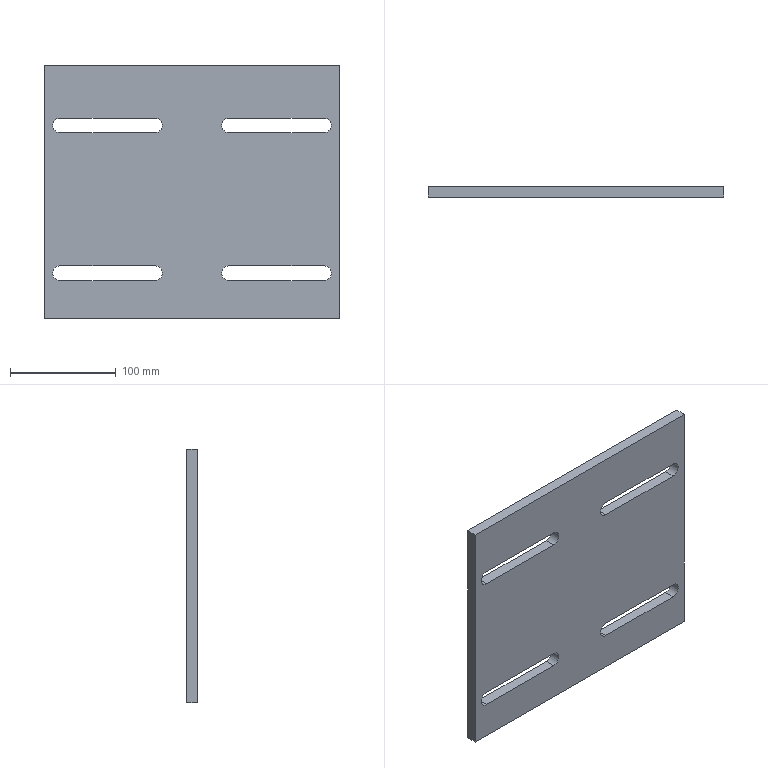Part | STEP file | Produce dryer line heating fan-motor base | 1 solid | 22 faces | box 280 x 10 x 240 mm | volume 615442 mm3 | plane 14 | cylinder 8 | commonest cylinder face diameters 14 x8
STEP:
#1=CARTESIAN_POINT('',(-125.,10.,70.));
#2=VERTEX_POINT('',#1);
#3=CARTESIAN_POINT('',(-35.,10.,70.));
#4=VERTEX_POINT('',#3);
#5=CARTESIAN_POINT('',(-125.,10.,70.));
#6=DIRECTION('',(1.,0.,0.));
#7=VECTOR('',#6,1000.);
#8=LINE('',#5,#7);
#9=EDGE_CURVE('',#2,#4,#8,.T.);
#10=ORIENTED_EDGE('',*,*,#9,.F.);
#11=CARTESIAN_POINT('',(-125.,10.,56.));
#12=VERTEX_POINT('',#11);
#13=CARTESIAN_POINT('',(-125.,10.,63.));
#14=DIRECTION('',(0.,1.,0.));
#15=DIRECTION('',(0.,0.,1.));
#16=AXIS2_PLACEMENT_3D('',#13,#14,#15);
#17=CIRCLE('',#16,7.);
#18=EDGE_CURVE('',#12,#2,#17,.T.);
#19=ORIENTED_EDGE('',*,*,#18,.F.);
#20=CARTESIAN_POINT('',(-35.,10.,56.));
#21=VERTEX_POINT('',#20);
#22=CARTESIAN_POINT('',(-125.,10.,56.));
#23=DIRECTION('',(-1.,0.,0.));
#24=VECTOR('',#23,1000.);
#25=LINE('',#22,#24);
#26=EDGE_CURVE('',#21,#12,#25,.T.);
#27=ORIENTED_EDGE('',*,*,#26,.F.);
#28=CARTESIAN_POINT('',(-35.,10.,63.));
#29=DIRECTION('',(0.,1.,0.));
#30=DIRECTION('',(0.,0.,1.));
#31=AXIS2_PLACEMENT_3D('',#28,#29,#30);
#32=CIRCLE('',#31,7.);
#33=EDGE_CURVE('',#4,#21,#32,.T.);
#34=ORIENTED_EDGE('',*,*,#33,.F.);
#35=EDGE_LOOP('',(#10,#19,#27,#34));
#36=FACE_BOUND('',#35,.T.);
#37=CARTESIAN_POINT('',(-125.,10.,-70.));
#38=VERTEX_POINT('',#37);
#39=CARTESIAN_POINT('',(-35.,10.,-70.));
#40=VERTEX_POINT('',#39);
#41=CARTESIAN_POINT('',(-125.,10.,-70.));
#42=DIRECTION('',(1.,0.,0.));
#43=VECTOR('',#42,1000.);
#44=LINE('',#41,#43);
#45=EDGE_CURVE('',#38,#40,#44,.T.);
#46=ORIENTED_EDGE('',*,*,#45,.F.);
#47=CARTESIAN_POINT('',(-125.,10.,-84.));
#48=VERTEX_POINT('',#47);
#49=CARTESIAN_POINT('',(-125.,10.,-77.));
#50=DIRECTION('',(0.,1.,0.));
#51=DIRECTION('',(0.,0.,1.));
#52=AXIS2_PLACEMENT_3D('',#49,#50,#51);
#53=CIRCLE('',#52,7.);
#54=EDGE_CURVE('',#48,#38,#53,.T.);
#55=ORIENTED_EDGE('',*,*,#54,.F.);
#56=CARTESIAN_POINT('',(-35.,10.,-84.));
#57=VERTEX_POINT('',#56);
#58=CARTESIAN_POINT('',(-125.,10.,-84.));
#59=DIRECTION('',(-1.,0.,0.));
#60=VECTOR('',#59,1000.);
#61=LINE('',#58,#60);
#62=EDGE_CURVE('',#57,#48,#61,.T.);
#63=ORIENTED_EDGE('',*,*,#62,.F.);
#64=CARTESIAN_POINT('',(-35.,10.,-77.));
#65=DIRECTION('',(0.,1.,0.));
#66=DIRECTION('',(0.,0.,1.));
#67=AXIS2_PLACEMENT_3D('',#64,#65,#66);
#68=CIRCLE('',#67,7.);
#69=EDGE_CURVE('',#40,#57,#68,.T.);
#70=ORIENTED_EDGE('',*,*,#69,.F.);
#71=EDGE_LOOP('',(#46,#55,#63,#70));
#72=FACE_BOUND('',#71,.T.);
#73=CARTESIAN_POINT('',(-140.,10.,-120.));
#74=VERTEX_POINT('',#73);
#75=CARTESIAN_POINT('',(-140.,10.,120.));
#76=VERTEX_POINT('',#75);
#77=CARTESIAN_POINT('',(-140.,10.,-120.));
#78=DIRECTION('',(0.,0.,1.));
#79=VECTOR('',#78,1000.);
#80=LINE('',#77,#79);
#81=EDGE_CURVE('',#74,#76,#80,.T.);
#82=ORIENTED_EDGE('',*,*,#81,.T.);
#83=CARTESIAN_POINT('',(140.,10.,120.));
#84=VERTEX_POINT('',#83);
#85=CARTESIAN_POINT('',(-140.,10.,120.));
#86=DIRECTION('',(1.,0.,0.));
#87=VECTOR('',#86,1000.);
#88=LINE('',#85,#87);
#89=EDGE_CURVE('',#76,#84,#88,.T.);
#90=ORIENTED_EDGE('',*,*,#89,.T.);
#91=CARTESIAN_POINT('',(140.,10.,-120.));
#92=VERTEX_POINT('',#91);
#93=CARTESIAN_POINT('',(140.,10.,-120.));
#94=DIRECTION('',(0.,0.,-1.));
#95=VECTOR('',#94,1000.);
#96=LINE('',#93,#95);
#97=EDGE_CURVE('',#84,#92,#96,.T.);
#98=ORIENTED_EDGE('',*,*,#97,.T.);
#99=CARTESIAN_POINT('',(-140.,10.,-120.));
#100=DIRECTION('',(-1.,0.,0.));
#101=VECTOR('',#100,1000.);
#102=LINE('',#99,#101);
#103=EDGE_CURVE('',#92,#74,#102,.T.);
#104=ORIENTED_EDGE('',*,*,#103,.T.);
#105=EDGE_LOOP('',(#82,#90,#98,#104));
#106=FACE_OUTER_BOUND('',#105,.T.);
#107=CARTESIAN_POINT('',(125.,10.,-84.));
#108=VERTEX_POINT('',#107);
#109=CARTESIAN_POINT('',(35.,10.,-84.));
#110=VERTEX_POINT('',#109);
#111=CARTESIAN_POINT('',(125.,10.,-84.));
#112=DIRECTION('',(-1.,0.,0.));
#113=VECTOR('',#112,1000.);
#114=LINE('',#111,#113);
#115=EDGE_CURVE('',#108,#110,#114,.T.);
#116=ORIENTED_EDGE('',*,*,#115,.F.);
#117=CARTESIAN_POINT('',(125.,10.,-70.));
#118=VERTEX_POINT('',#117);
#119=CARTESIAN_POINT('',(125.,10.,-77.));
#120=DIRECTION('',(0.,1.,0.));
#121=DIRECTION('',(0.,0.,1.));
#122=AXIS2_PLACEMENT_3D('',#119,#120,#121);
#123=CIRCLE('',#122,7.);
#124=EDGE_CURVE('',#118,#108,#123,.T.);
#125=ORIENTED_EDGE('',*,*,#124,.F.);
#126=CARTESIAN_POINT('',(35.,10.,-70.));
#127=VERTEX_POINT('',#126);
#128=CARTESIAN_POINT('',(125.,10.,-70.));
#129=DIRECTION('',(1.,0.,0.));
#130=VECTOR('',#129,1000.);
#131=LINE('',#128,#130);
#132=EDGE_CURVE('',#127,#118,#131,.T.);
#133=ORIENTED_EDGE('',*,*,#132,.F.);
#134=CARTESIAN_POINT('',(35.,10.,-77.));
#135=DIRECTION('',(0.,1.,0.));
#136=DIRECTION('',(0.,0.,1.));
#137=AXIS2_PLACEMENT_3D('',#134,#135,#136);
#138=CIRCLE('',#137,7.);
#139=EDGE_CURVE('',#110,#127,#138,.T.);
#140=ORIENTED_EDGE('',*,*,#139,.F.);
#141=EDGE_LOOP('',(#116,#125,#133,#140));
#142=FACE_BOUND('',#141,.T.);
#143=CARTESIAN_POINT('',(35.,10.,70.));
#144=VERTEX_POINT('',#143);
#145=CARTESIAN_POINT('',(125.,10.,70.));
#146=VERTEX_POINT('',#145);
#147=CARTESIAN_POINT('',(35.,10.,70.));
#148=DIRECTION('',(1.,0.,0.));
#149=VECTOR('',#148,1000.);
#150=LINE('',#147,#149);
#151=EDGE_CURVE('',#144,#146,#150,.T.);
#152=ORIENTED_EDGE('',*,*,#151,.F.);
#153=CARTESIAN_POINT('',(35.,10.,56.));
#154=VERTEX_POINT('',#153);
#155=CARTESIAN_POINT('',(35.,10.,63.));
#156=DIRECTION('',(0.,1.,0.));
#157=DIRECTION('',(0.,0.,1.));
#158=AXIS2_PLACEMENT_3D('',#155,#156,#157);
#159=CIRCLE('',#158,7.);
#160=EDGE_CURVE('',#154,#144,#159,.T.);
#161=ORIENTED_EDGE('',*,*,#160,.F.);
#162=CARTESIAN_POINT('',(125.,10.,56.));
#163=VERTEX_POINT('',#162);
#164=CARTESIAN_POINT('',(35.,10.,56.));
#165=DIRECTION('',(-1.,0.,0.));
#166=VECTOR('',#165,1000.);
#167=LINE('',#164,#166);
#168=EDGE_CURVE('',#163,#154,#167,.T.);
#169=ORIENTED_EDGE('',*,*,#168,.F.);
#170=CARTESIAN_POINT('',(125.,10.,63.));
#171=DIRECTION('',(0.,1.,0.));
#172=DIRECTION('',(0.,0.,1.));
#173=AXIS2_PLACEMENT_3D('',#170,#171,#172);
#174=CIRCLE('',#173,7.);
#175=EDGE_CURVE('',#146,#163,#174,.T.);
#176=ORIENTED_EDGE('',*,*,#175,.F.);
#177=EDGE_LOOP('',(#152,#161,#169,#176));
#178=FACE_BOUND('',#177,.T.);
#179=CARTESIAN_POINT('',(-140.,10.,120.));
#180=DIRECTION('',(0.,1.,0.));
#181=DIRECTION('',(0.,0.,1.));
#182=AXIS2_PLACEMENT_3D('',#179,#180,#181);
#183=PLANE('',#182);
#184=ADVANCED_FACE('',(#36,#72,#106,#142,#178),#183,.T.);
#185=CARTESIAN_POINT('',(-125.,0.,56.));
#186=VERTEX_POINT('',#185);
#187=CARTESIAN_POINT('',(-125.,0.,70.));
#188=VERTEX_POINT('',#187);
#189=CARTESIAN_POINT('',(-125.,0.,63.));
#190=DIRECTION('',(0.,1.,0.));
#191=DIRECTION('',(0.,0.,1.));
#192=AXIS2_PLACEMENT_3D('',#189,#190,#191);
#193=CIRCLE('',#192,7.);
#194=EDGE_CURVE('',#186,#188,#193,.T.);
#195=ORIENTED_EDGE('',*,*,#194,.T.);
#196=CARTESIAN_POINT('',(-35.,0.,70.));
#197=VERTEX_POINT('',#196);
#198=CARTESIAN_POINT('',(-125.,0.,70.));
#199=DIRECTION('',(1.,0.,0.));
#200=VECTOR('',#199,1000.);
#201=LINE('',#198,#200);
#202=EDGE_CURVE('',#188,#197,#201,.T.);
#203=ORIENTED_EDGE('',*,*,#202,.T.);
#204=CARTESIAN_POINT('',(-35.,0.,56.));
#205=VERTEX_POINT('',#204);
#206=CARTESIAN_POINT('',(-35.,0.,63.));
#207=DIRECTION('',(0.,1.,0.));
#208=DIRECTION('',(0.,0.,1.));
#209=AXIS2_PLACEMENT_3D('',#206,#207,#208);
#210=CIRCLE('',#209,7.);
#211=EDGE_CURVE('',#197,#205,#210,.T.);
#212=ORIENTED_EDGE('',*,*,#211,.T.);
#213=CARTESIAN_POINT('',(-125.,0.,56.));
#214=DIRECTION('',(-1.,0.,0.));
#215=VECTOR('',#214,1000.);
#216=LINE('',#213,#215);
#217=EDGE_CURVE('',#205,#186,#216,.T.);
#218=ORIENTED_EDGE('',*,*,#217,.T.);
#219=EDGE_LOOP('',(#195,#203,#212,#218));
#220=FACE_BOUND('',#219,.T.);
#221=CARTESIAN_POINT('',(-125.,0.,-84.));
#222=VERTEX_POINT('',#221);
#223=CARTESIAN_POINT('',(-125.,0.,-70.));
#224=VERTEX_POINT('',#223);
#225=CARTESIAN_POINT('',(-125.,0.,-77.));
#226=DIRECTION('',(0.,1.,0.));
#227=DIRECTION('',(0.,0.,1.));
#228=AXIS2_PLACEMENT_3D('',#225,#226,#227);
#229=CIRCLE('',#228,7.);
#230=EDGE_CURVE('',#222,#224,#229,.T.);
#231=ORIENTED_EDGE('',*,*,#230,.T.);
#232=CARTESIAN_POINT('',(-35.,0.,-70.));
#233=VERTEX_POINT('',#232);
#234=CARTESIAN_POINT('',(-125.,0.,-70.));
#235=DIRECTION('',(1.,0.,0.));
#236=VECTOR('',#235,1000.);
#237=LINE('',#234,#236);
#238=EDGE_CURVE('',#224,#233,#237,.T.);
#239=ORIENTED_EDGE('',*,*,#238,.T.);
#240=CARTESIAN_POINT('',(-35.,0.,-84.));
#241=VERTEX_POINT('',#240);
#242=CARTESIAN_POINT('',(-35.,0.,-77.));
#243=DIRECTION('',(0.,1.,0.));
#244=DIRECTION('',(0.,0.,1.));
#245=AXIS2_PLACEMENT_3D('',#242,#243,#244);
#246=CIRCLE('',#245,7.);
#247=EDGE_CURVE('',#233,#241,#246,.T.);
#248=ORIENTED_EDGE('',*,*,#247,.T.);
#249=CARTESIAN_POINT('',(-125.,0.,-84.));
#250=DIRECTION('',(-1.,0.,0.));
#251=VECTOR('',#250,1000.);
#252=LINE('',#249,#251);
#253=EDGE_CURVE('',#241,#222,#252,.T.);
#254=ORIENTED_EDGE('',*,*,#253,.T.);
#255=EDGE_LOOP('',(#231,#239,#248,#254));
#256=FACE_BOUND('',#255,.T.);
#257=CARTESIAN_POINT('',(-140.,0.,-120.));
#258=VERTEX_POINT('',#257);
#259=CARTESIAN_POINT('',(-140.,0.,120.));
#260=VERTEX_POINT('',#259);
#261=CARTESIAN_POINT('',(-140.,0.,-120.));
#262=DIRECTION('',(0.,0.,1.));
#263=VECTOR('',#262,1000.);
#264=LINE('',#261,#263);
#265=EDGE_CURVE('',#258,#260,#264,.T.);
#266=ORIENTED_EDGE('',*,*,#265,.F.);
#267=CARTESIAN_POINT('',(140.,0.,-120.));
#268=VERTEX_POINT('',#267);
#269=CARTESIAN_POINT('',(-140.,0.,-120.));
#270=DIRECTION('',(-1.,0.,0.));
#271=VECTOR('',#270,1000.);
#272=LINE('',#269,#271);
#273=EDGE_CURVE('',#268,#258,#272,.T.);
#274=ORIENTED_EDGE('',*,*,#273,.F.);
#275=CARTESIAN_POINT('',(140.,0.,120.));
#276=VERTEX_POINT('',#275);
#277=CARTESIAN_POINT('',(140.,0.,-120.));
#278=DIRECTION('',(0.,0.,-1.));
#279=VECTOR('',#278,1000.);
#280=LINE('',#277,#279);
#281=EDGE_CURVE('',#276,#268,#280,.T.);
#282=ORIENTED_EDGE('',*,*,#281,.F.);
#283=CARTESIAN_POINT('',(-140.,0.,120.));
#284=DIRECTION('',(1.,0.,0.));
#285=VECTOR('',#284,1000.);
#286=LINE('',#283,#285);
#287=EDGE_CURVE('',#260,#276,#286,.T.);
#288=ORIENTED_EDGE('',*,*,#287,.F.);
#289=EDGE_LOOP('',(#266,#274,#282,#288));
#290=FACE_OUTER_BOUND('',#289,.T.);
#291=CARTESIAN_POINT('',(125.,0.,-70.));
#292=VERTEX_POINT('',#291);
#293=CARTESIAN_POINT('',(125.,0.,-84.));
#294=VERTEX_POINT('',#293);
#295=CARTESIAN_POINT('',(125.,0.,-77.));
#296=DIRECTION('',(0.,1.,0.));
#297=DIRECTION('',(0.,0.,1.));
#298=AXIS2_PLACEMENT_3D('',#295,#296,#297);
#299=CIRCLE('',#298,7.);
#300=EDGE_CURVE('',#292,#294,#299,.T.);
#301=ORIENTED_EDGE('',*,*,#300,.T.);
#302=CARTESIAN_POINT('',(35.,0.,-84.));
#303=VERTEX_POINT('',#302);
#304=CARTESIAN_POINT('',(125.,0.,-84.));
#305=DIRECTION('',(-1.,0.,0.));
#306=VECTOR('',#305,1000.);
#307=LINE('',#304,#306);
#308=EDGE_CURVE('',#294,#303,#307,.T.);
#309=ORIENTED_EDGE('',*,*,#308,.T.);
#310=CARTESIAN_POINT('',(35.,0.,-70.));
#311=VERTEX_POINT('',#310);
#312=CARTESIAN_POINT('',(35.,0.,-77.));
#313=DIRECTION('',(0.,1.,0.));
#314=DIRECTION('',(0.,0.,1.));
#315=AXIS2_PLACEMENT_3D('',#312,#313,#314);
#316=CIRCLE('',#315,7.);
#317=EDGE_CURVE('',#303,#311,#316,.T.);
#318=ORIENTED_EDGE('',*,*,#317,.T.);
#319=CARTESIAN_POINT('',(125.,0.,-70.));
#320=DIRECTION('',(1.,0.,0.));
#321=VECTOR('',#320,1000.);
#322=LINE('',#319,#321);
#323=EDGE_CURVE('',#311,#292,#322,.T.);
#324=ORIENTED_EDGE('',*,*,#323,.T.);
#325=EDGE_LOOP('',(#301,#309,#318,#324));
#326=FACE_BOUND('',#325,.T.);
#327=CARTESIAN_POINT('',(35.,0.,56.));
#328=VERTEX_POINT('',#327);
#329=CARTESIAN_POINT('',(35.,0.,70.));
#330=VERTEX_POINT('',#329);
#331=CARTESIAN_POINT('',(35.,0.,63.));
#332=DIRECTION('',(0.,1.,0.));
#333=DIRECTION('',(0.,0.,1.));
#334=AXIS2_PLACEMENT_3D('',#331,#332,#333);
#335=CIRCLE('',#334,7.);
#336=EDGE_CURVE('',#328,#330,#335,.T.);
#337=ORIENTED_EDGE('',*,*,#336,.T.);
#338=CARTESIAN_POINT('',(125.,0.,70.));
#339=VERTEX_POINT('',#338);
#340=CARTESIAN_POINT('',(35.,0.,70.));
#341=DIRECTION('',(1.,0.,0.));
#342=VECTOR('',#341,1000.);
#343=LINE('',#340,#342);
#344=EDGE_CURVE('',#330,#339,#343,.T.);
#345=ORIENTED_EDGE('',*,*,#344,.T.);
#346=CARTESIAN_POINT('',(125.,0.,56.));
#347=VERTEX_POINT('',#346);
#348=CARTESIAN_POINT('',(125.,0.,63.));
#349=DIRECTION('',(0.,1.,0.));
#350=DIRECTION('',(0.,0.,1.));
#351=AXIS2_PLACEMENT_3D('',#348,#349,#350);
#352=CIRCLE('',#351,7.);
#353=EDGE_CURVE('',#339,#347,#352,.T.);
#354=ORIENTED_EDGE('',*,*,#353,.T.);
#355=CARTESIAN_POINT('',(35.,0.,56.));
#356=DIRECTION('',(-1.,0.,0.));
#357=VECTOR('',#356,1000.);
#358=LINE('',#355,#357);
#359=EDGE_CURVE('',#347,#328,#358,.T.);
#360=ORIENTED_EDGE('',*,*,#359,.T.);
#361=EDGE_LOOP('',(#337,#345,#354,#360));
#362=FACE_BOUND('',#361,.T.);
#363=CARTESIAN_POINT('',(-140.,0.,120.));
#364=DIRECTION('',(0.,1.,0.));
#365=DIRECTION('',(0.,0.,1.));
#366=AXIS2_PLACEMENT_3D('',#363,#364,#365);
#367=PLANE('',#366);
#368=ADVANCED_FACE('',(#220,#256,#290,#326,#362),#367,.F.);
#369=ORIENTED_EDGE('',*,*,#265,.T.);
#370=CARTESIAN_POINT('',(-140.,10.,120.));
#371=DIRECTION('',(0.,-1.,0.));
#372=VECTOR('',#371,1000.);
#373=LINE('',#370,#372);
#374=EDGE_CURVE('',#76,#260,#373,.T.);
#375=ORIENTED_EDGE('',*,*,#374,.F.);
#376=ORIENTED_EDGE('',*,*,#81,.F.);
#377=CARTESIAN_POINT('',(-140.,10.,-120.));
#378=DIRECTION('',(0.,-1.,0.));
#379=VECTOR('',#378,1000.);
#380=LINE('',#377,#379);
#381=EDGE_CURVE('',#74,#258,#380,.T.);
#382=ORIENTED_EDGE('',*,*,#381,.T.);
#383=EDGE_LOOP('',(#369,#375,#376,#382));
#384=FACE_OUTER_BOUND('',#383,.T.);
#385=CARTESIAN_POINT('',(-140.,10.,-120.));
#386=DIRECTION('',(1.,0.,0.));
#387=DIRECTION('',(0.,0.,-1.));
#388=AXIS2_PLACEMENT_3D('',#385,#386,#387);
#389=PLANE('',#388);
#390=ADVANCED_FACE('',(#384),#389,.F.);
#391=ORIENTED_EDGE('',*,*,#287,.T.);
#392=CARTESIAN_POINT('',(140.,10.,120.));
#393=DIRECTION('',(0.,-1.,0.));
#394=VECTOR('',#393,1000.);
#395=LINE('',#392,#394);
#396=EDGE_CURVE('',#84,#276,#395,.T.);
#397=ORIENTED_EDGE('',*,*,#396,.F.);
#398=ORIENTED_EDGE('',*,*,#89,.F.);
#399=ORIENTED_EDGE('',*,*,#374,.T.);
#400=EDGE_LOOP('',(#391,#397,#398,#399));
#401=FACE_OUTER_BOUND('',#400,.T.);
#402=CARTESIAN_POINT('',(-140.,10.,120.));
#403=DIRECTION('',(0.,0.,-1.));
#404=DIRECTION('',(-1.,0.,0.));
#405=AXIS2_PLACEMENT_3D('',#402,#403,#404);
#406=PLANE('',#405);
#407=ADVANCED_FACE('',(#401),#406,.F.);
#408=ORIENTED_EDGE('',*,*,#281,.T.);
#409=CARTESIAN_POINT('',(140.,10.,-120.));
#410=DIRECTION('',(0.,-1.,0.));
#411=VECTOR('',#410,1000.);
#412=LINE('',#409,#411);
#413=EDGE_CURVE('',#92,#268,#412,.T.);
#414=ORIENTED_EDGE('',*,*,#413,.F.);
#415=ORIENTED_EDGE('',*,*,#97,.F.);
#416=ORIENTED_EDGE('',*,*,#396,.T.);
#417=EDGE_LOOP('',(#408,#414,#415,#416));
#418=FACE_OUTER_BOUND('',#417,.T.);
#419=CARTESIAN_POINT('',(140.,10.,-120.));
#420=DIRECTION('',(-1.,0.,0.));
#421=DIRECTION('',(0.,0.,1.));
#422=AXIS2_PLACEMENT_3D('',#419,#420,#421);
#423=PLANE('',#422);
#424=ADVANCED_FACE('',(#418),#423,.F.);
#425=ORIENTED_EDGE('',*,*,#273,.T.);
#426=ORIENTED_EDGE('',*,*,#381,.F.);
#427=ORIENTED_EDGE('',*,*,#103,.F.);
#428=ORIENTED_EDGE('',*,*,#413,.T.);
#429=EDGE_LOOP('',(#425,#426,#427,#428));
#430=FACE_OUTER_BOUND('',#429,.T.);
#431=CARTESIAN_POINT('',(-140.,10.,-120.));
#432=DIRECTION('',(0.,0.,1.));
#433=DIRECTION('',(1.,0.,0.));
#434=AXIS2_PLACEMENT_3D('',#431,#432,#433);
#435=PLANE('',#434);
#436=ADVANCED_FACE('',(#430),#435,.F.);
#437=ORIENTED_EDGE('',*,*,#230,.F.);
#438=CARTESIAN_POINT('',(-125.,10.,-84.));
#439=DIRECTION('',(0.,-1.,0.));
#440=VECTOR('',#439,1000.);
#441=LINE('',#438,#440);
#442=EDGE_CURVE('',#48,#222,#441,.T.);
#443=ORIENTED_EDGE('',*,*,#442,.F.);
#444=ORIENTED_EDGE('',*,*,#54,.T.);
#445=CARTESIAN_POINT('',(-125.,10.,-70.));
#446=DIRECTION('',(0.,-1.,0.));
#447=VECTOR('',#446,1000.);
#448=LINE('',#445,#447);
#449=EDGE_CURVE('',#38,#224,#448,.T.);
#450=ORIENTED_EDGE('',*,*,#449,.T.);
#451=EDGE_LOOP('',(#437,#443,#444,#450));
#452=FACE_OUTER_BOUND('',#451,.T.);
#453=CARTESIAN_POINT('',(-125.,10.,-77.));
#454=DIRECTION('',(0.,-1.,0.));
#455=DIRECTION('',(0.,0.,-1.));
#456=AXIS2_PLACEMENT_3D('',#453,#454,#455);
#457=CYLINDRICAL_SURFACE('',#456,7.);
#458=ADVANCED_FACE('',(#452),#457,.F.);
#459=ORIENTED_EDGE('',*,*,#238,.F.);
#460=ORIENTED_EDGE('',*,*,#449,.F.);
#461=ORIENTED_EDGE('',*,*,#45,.T.);
#462=CARTESIAN_POINT('',(-35.,10.,-70.));
#463=DIRECTION('',(0.,-1.,0.));
#464=VECTOR('',#463,1000.);
#465=LINE('',#462,#464);
#466=EDGE_CURVE('',#40,#233,#465,.T.);
#467=ORIENTED_EDGE('',*,*,#466,.T.);
#468=EDGE_LOOP('',(#459,#460,#461,#467));
#469=FACE_OUTER_BOUND('',#468,.T.);
#470=CARTESIAN_POINT('',(-125.,10.,-70.));
#471=DIRECTION('',(0.,0.,-1.));
#472=DIRECTION('',(-1.,0.,0.));
#473=AXIS2_PLACEMENT_3D('',#470,#471,#472);
#474=PLANE('',#473);
#475=ADVANCED_FACE('',(#469),#474,.T.);
#476=ORIENTED_EDGE('',*,*,#247,.F.);
#477=ORIENTED_EDGE('',*,*,#466,.F.);
#478=ORIENTED_EDGE('',*,*,#69,.T.);
#479=CARTESIAN_POINT('',(-35.,10.,-84.));
#480=DIRECTION('',(0.,-1.,0.));
#481=VECTOR('',#480,1000.);
#482=LINE('',#479,#481);
#483=EDGE_CURVE('',#57,#241,#482,.T.);
#484=ORIENTED_EDGE('',*,*,#483,.T.);
#485=EDGE_LOOP('',(#476,#477,#478,#484));
#486=FACE_OUTER_BOUND('',#485,.T.);
#487=CARTESIAN_POINT('',(-35.,10.,-77.));
#488=DIRECTION('',(0.,-1.,0.));
#489=DIRECTION('',(0.,0.,-1.));
#490=AXIS2_PLACEMENT_3D('',#487,#488,#489);
#491=CYLINDRICAL_SURFACE('',#490,7.);
#492=ADVANCED_FACE('',(#486),#491,.F.);
#493=ORIENTED_EDGE('',*,*,#253,.F.);
#494=ORIENTED_EDGE('',*,*,#483,.F.);
#495=ORIENTED_EDGE('',*,*,#62,.T.);
#496=ORIENTED_EDGE('',*,*,#442,.T.);
#497=EDGE_LOOP('',(#493,#494,#495,#496));
#498=FACE_OUTER_BOUND('',#497,.T.);
#499=CARTESIAN_POINT('',(-125.,10.,-84.));
#500=DIRECTION('',(0.,0.,1.));
#501=DIRECTION('',(1.,0.,0.));
#502=AXIS2_PLACEMENT_3D('',#499,#500,#501);
#503=PLANE('',#502);
#504=ADVANCED_FACE('',(#498),#503,.T.);
#505=ORIENTED_EDGE('',*,*,#300,.F.);
#506=CARTESIAN_POINT('',(125.,10.,-70.));
#507=DIRECTION('',(0.,-1.,0.));
#508=VECTOR('',#507,1000.);
#509=LINE('',#506,#508);
#510=EDGE_CURVE('',#118,#292,#509,.T.);
#511=ORIENTED_EDGE('',*,*,#510,.F.);
#512=ORIENTED_EDGE('',*,*,#124,.T.);
#513=CARTESIAN_POINT('',(125.,10.,-84.));
#514=DIRECTION('',(0.,-1.,0.));
#515=VECTOR('',#514,1000.);
#516=LINE('',#513,#515);
#517=EDGE_CURVE('',#108,#294,#516,.T.);
#518=ORIENTED_EDGE('',*,*,#517,.T.);
#519=EDGE_LOOP('',(#505,#511,#512,#518));
#520=FACE_OUTER_BOUND('',#519,.T.);
#521=CARTESIAN_POINT('',(125.,10.,-77.));
#522=DIRECTION('',(0.,-1.,0.));
#523=DIRECTION('',(0.,0.,-1.));
#524=AXIS2_PLACEMENT_3D('',#521,#522,#523);
#525=CYLINDRICAL_SURFACE('',#524,7.);
#526=ADVANCED_FACE('',(#520),#525,.F.);
#527=ORIENTED_EDGE('',*,*,#308,.F.);
#528=ORIENTED_EDGE('',*,*,#517,.F.);
#529=ORIENTED_EDGE('',*,*,#115,.T.);
#530=CARTESIAN_POINT('',(35.,10.,-84.));
#531=DIRECTION('',(0.,-1.,0.));
#532=VECTOR('',#531,1000.);
#533=LINE('',#530,#532);
#534=EDGE_CURVE('',#110,#303,#533,.T.);
#535=ORIENTED_EDGE('',*,*,#534,.T.);
#536=EDGE_LOOP('',(#527,#528,#529,#535));
#537=FACE_OUTER_BOUND('',#536,.T.);
#538=CARTESIAN_POINT('',(125.,10.,-84.));
#539=DIRECTION('',(0.,0.,1.));
#540=DIRECTION('',(1.,0.,0.));
#541=AXIS2_PLACEMENT_3D('',#538,#539,#540);
#542=PLANE('',#541);
#543=ADVANCED_FACE('',(#537),#542,.T.);
#544=ORIENTED_EDGE('',*,*,#317,.F.);
#545=ORIENTED_EDGE('',*,*,#534,.F.);
#546=ORIENTED_EDGE('',*,*,#139,.T.);
#547=CARTESIAN_POINT('',(35.,10.,-70.));
#548=DIRECTION('',(0.,-1.,0.));
#549=VECTOR('',#548,1000.);
#550=LINE('',#547,#549);
#551=EDGE_CURVE('',#127,#311,#550,.T.);
#552=ORIENTED_EDGE('',*,*,#551,.T.);
#553=EDGE_LOOP('',(#544,#545,#546,#552));
#554=FACE_OUTER_BOUND('',#553,.T.);
#555=CARTESIAN_POINT('',(35.,10.,-77.));
#556=DIRECTION('',(0.,-1.,0.));
#557=DIRECTION('',(0.,0.,-1.));
#558=AXIS2_PLACEMENT_3D('',#555,#556,#557);
#559=CYLINDRICAL_SURFACE('',#558,7.);
#560=ADVANCED_FACE('',(#554),#559,.F.);
#561=ORIENTED_EDGE('',*,*,#323,.F.);
#562=ORIENTED_EDGE('',*,*,#551,.F.);
#563=ORIENTED_EDGE('',*,*,#132,.T.);
#564=ORIENTED_EDGE('',*,*,#510,.T.);
#565=EDGE_LOOP('',(#561,#562,#563,#564));
#566=FACE_OUTER_BOUND('',#565,.T.);
#567=CARTESIAN_POINT('',(125.,10.,-70.));
#568=DIRECTION('',(0.,0.,-1.));
#569=DIRECTION('',(-1.,0.,0.));
#570=AXIS2_PLACEMENT_3D('',#567,#568,#569);
#571=PLANE('',#570);
#572=ADVANCED_FACE('',(#566),#571,.T.);
#573=ORIENTED_EDGE('',*,*,#194,.F.);
#574=CARTESIAN_POINT('',(-125.,10.,56.));
#575=DIRECTION('',(0.,-1.,0.));
#576=VECTOR('',#575,1000.);
#577=LINE('',#574,#576);
#578=EDGE_CURVE('',#12,#186,#577,.T.);
#579=ORIENTED_EDGE('',*,*,#578,.F.);
#580=ORIENTED_EDGE('',*,*,#18,.T.);
#581=CARTESIAN_POINT('',(-125.,10.,70.));
#582=DIRECTION('',(0.,-1.,0.));
#583=VECTOR('',#582,1000.);
#584=LINE('',#581,#583);
#585=EDGE_CURVE('',#2,#188,#584,.T.);
#586=ORIENTED_EDGE('',*,*,#585,.T.);
#587=EDGE_LOOP('',(#573,#579,#580,#586));
#588=FACE_OUTER_BOUND('',#587,.T.);
#589=CARTESIAN_POINT('',(-125.,10.,63.));
#590=DIRECTION('',(0.,-1.,0.));
#591=DIRECTION('',(0.,0.,-1.));
#592=AXIS2_PLACEMENT_3D('',#589,#590,#591);
#593=CYLINDRICAL_SURFACE('',#592,7.);
#594=ADVANCED_FACE('',(#588),#593,.F.);
#595=ORIENTED_EDGE('',*,*,#202,.F.);
#596=ORIENTED_EDGE('',*,*,#585,.F.);
#597=ORIENTED_EDGE('',*,*,#9,.T.);
#598=CARTESIAN_POINT('',(-35.,10.,70.));
#599=DIRECTION('',(0.,-1.,0.));
#600=VECTOR('',#599,1000.);
#601=LINE('',#598,#600);
#602=EDGE_CURVE('',#4,#197,#601,.T.);
#603=ORIENTED_EDGE('',*,*,#602,.T.);
#604=EDGE_LOOP('',(#595,#596,#597,#603));
#605=FACE_OUTER_BOUND('',#604,.T.);
#606=CARTESIAN_POINT('',(-125.,10.,70.));
#607=DIRECTION('',(0.,0.,-1.));
#608=DIRECTION('',(-1.,0.,0.));
#609=AXIS2_PLACEMENT_3D('',#606,#607,#608);
#610=PLANE('',#609);
#611=ADVANCED_FACE('',(#605),#610,.T.);
#612=ORIENTED_EDGE('',*,*,#211,.F.);
#613=ORIENTED_EDGE('',*,*,#602,.F.);
#614=ORIENTED_EDGE('',*,*,#33,.T.);
#615=CARTESIAN_POINT('',(-35.,10.,56.));
#616=DIRECTION('',(0.,-1.,0.));
#617=VECTOR('',#616,1000.);
#618=LINE('',#615,#617);
#619=EDGE_CURVE('',#21,#205,#618,.T.);
#620=ORIENTED_EDGE('',*,*,#619,.T.);
#621=EDGE_LOOP('',(#612,#613,#614,#620));
#622=FACE_OUTER_BOUND('',#621,.T.);
#623=CARTESIAN_POINT('',(-35.,10.,63.));
#624=DIRECTION('',(0.,-1.,0.));
#625=DIRECTION('',(0.,0.,-1.));
#626=AXIS2_PLACEMENT_3D('',#623,#624,#625);
#627=CYLINDRICAL_SURFACE('',#626,7.);
#628=ADVANCED_FACE('',(#622),#627,.F.);
#629=ORIENTED_EDGE('',*,*,#217,.F.);
#630=ORIENTED_EDGE('',*,*,#619,.F.);
#631=ORIENTED_EDGE('',*,*,#26,.T.);
#632=ORIENTED_EDGE('',*,*,#578,.T.);
#633=EDGE_LOOP('',(#629,#630,#631,#632));
#634=FACE_OUTER_BOUND('',#633,.T.);
#635=CARTESIAN_POINT('',(-125.,10.,56.));
#636=DIRECTION('',(0.,0.,1.));
#637=DIRECTION('',(1.,0.,0.));
#638=AXIS2_PLACEMENT_3D('',#635,#636,#637);
#639=PLANE('',#638);
#640=ADVANCED_FACE('',(#634),#639,.T.);
#641=ORIENTED_EDGE('',*,*,#336,.F.);
#642=CARTESIAN_POINT('',(35.,10.,56.));
#643=DIRECTION('',(0.,-1.,0.));
#644=VECTOR('',#643,1000.);
#645=LINE('',#642,#644);
#646=EDGE_CURVE('',#154,#328,#645,.T.);
#647=ORIENTED_EDGE('',*,*,#646,.F.);
#648=ORIENTED_EDGE('',*,*,#160,.T.);
#649=CARTESIAN_POINT('',(35.,10.,70.));
#650=DIRECTION('',(0.,-1.,0.));
#651=VECTOR('',#650,1000.);
#652=LINE('',#649,#651);
#653=EDGE_CURVE('',#144,#330,#652,.T.);
#654=ORIENTED_EDGE('',*,*,#653,.T.);
#655=EDGE_LOOP('',(#641,#647,#648,#654));
#656=FACE_OUTER_BOUND('',#655,.T.);
#657=CARTESIAN_POINT('',(35.,10.,63.));
#658=DIRECTION('',(0.,-1.,0.));
#659=DIRECTION('',(0.,0.,-1.));
#660=AXIS2_PLACEMENT_3D('',#657,#658,#659);
#661=CYLINDRICAL_SURFACE('',#660,7.);
#662=ADVANCED_FACE('',(#656),#661,.F.);
#663=ORIENTED_EDGE('',*,*,#344,.F.);
#664=ORIENTED_EDGE('',*,*,#653,.F.);
#665=ORIENTED_EDGE('',*,*,#151,.T.);
#666=CARTESIAN_POINT('',(125.,10.,70.));
#667=DIRECTION('',(0.,-1.,0.));
#668=VECTOR('',#667,1000.);
#669=LINE('',#666,#668);
#670=EDGE_CURVE('',#146,#339,#669,.T.);
#671=ORIENTED_EDGE('',*,*,#670,.T.);
#672=EDGE_LOOP('',(#663,#664,#665,#671));
#673=FACE_OUTER_BOUND('',#672,.T.);
#674=CARTESIAN_POINT('',(35.,10.,70.));
#675=DIRECTION('',(0.,0.,-1.));
#676=DIRECTION('',(-1.,0.,0.));
#677=AXIS2_PLACEMENT_3D('',#674,#675,#676);
#678=PLANE('',#677);
#679=ADVANCED_FACE('',(#673),#678,.T.);
#680=ORIENTED_EDGE('',*,*,#353,.F.);
#681=ORIENTED_EDGE('',*,*,#670,.F.);
#682=ORIENTED_EDGE('',*,*,#175,.T.);
#683=CARTESIAN_POINT('',(125.,10.,56.));
#684=DIRECTION('',(0.,-1.,0.));
#685=VECTOR('',#684,1000.);
#686=LINE('',#683,#685);
#687=EDGE_CURVE('',#163,#347,#686,.T.);
#688=ORIENTED_EDGE('',*,*,#687,.T.);
#689=EDGE_LOOP('',(#680,#681,#682,#688));
#690=FACE_OUTER_BOUND('',#689,.T.);
#691=CARTESIAN_POINT('',(125.,10.,63.));
#692=DIRECTION('',(0.,-1.,0.));
#693=DIRECTION('',(0.,0.,-1.));
#694=AXIS2_PLACEMENT_3D('',#691,#692,#693);
#695=CYLINDRICAL_SURFACE('',#694,7.);
#696=ADVANCED_FACE('',(#690),#695,.F.);
#697=ORIENTED_EDGE('',*,*,#359,.F.);
#698=ORIENTED_EDGE('',*,*,#687,.F.);
#699=ORIENTED_EDGE('',*,*,#168,.T.);
#700=ORIENTED_EDGE('',*,*,#646,.T.);
#701=EDGE_LOOP('',(#697,#698,#699,#700));
#702=FACE_OUTER_BOUND('',#701,.T.);
#703=CARTESIAN_POINT('',(35.,10.,56.));
#704=DIRECTION('',(0.,0.,1.));
#705=DIRECTION('',(1.,0.,0.));
#706=AXIS2_PLACEMENT_3D('',#703,#704,#705);
#707=PLANE('',#706);
#708=ADVANCED_FACE('',(#702),#707,.T.);
#709=CLOSED_SHELL('',(#184,#368,#390,#407,#424,#436,#458,#475,#492,#504,#526,#543,#560,#572,#594,#611,#628,#640,#662,#679,#696,#708));
#710=MANIFOLD_SOLID_BREP('',#709);
#711=CARTESIAN_POINT('',(0.,0.,0.));
#712=DIRECTION('',(0.,0.,1.));
#713=DIRECTION('',(1.,0.,0.));
#714=AXIS2_PLACEMENT_3D('',#711,#712,#713);
#715=(LENGTH_UNIT()NAMED_UNIT(*)SI_UNIT(.MILLI.,.METRE.));
#716=UNCERTAINTY_MEASURE_WITH_UNIT(LENGTH_MEASURE(0.00001),#715,'','');
#717=(NAMED_UNIT(*)PLANE_ANGLE_UNIT()SI_UNIT($,.RADIAN.));
#718=(NAMED_UNIT(*)SI_UNIT($,.STERADIAN.)SOLID_ANGLE_UNIT());
#719=(GEOMETRIC_REPRESENTATION_CONTEXT(3)GLOBAL_UNCERTAINTY_ASSIGNED_CONTEXT((#716))GLOBAL_UNIT_ASSIGNED_CONTEXT((#715,#717,#718))REPRESENTATION_CONTEXT('',''));
#720=ADVANCED_BREP_SHAPE_REPRESENTATION('',(#710,#714),#719);